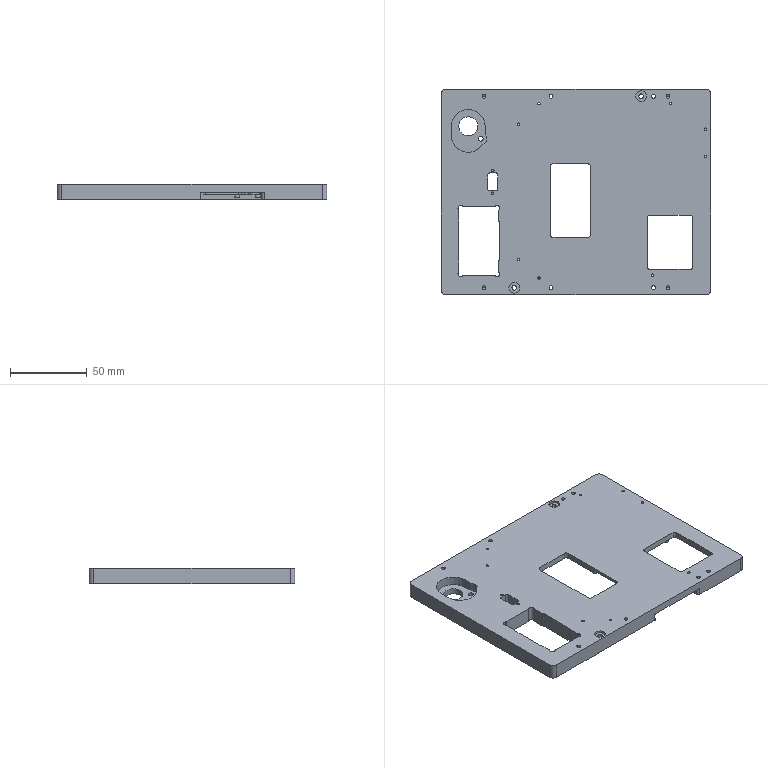NC program | NX | posted with a generic post | part box 176 x 134 x 10 mm
Lines 2298 to 3227 of 17594:
(CAVITY_MILL_COPY , TOOL : D6JING)
N4582 T16 M6
N4584 G54
N4586 G17 G0 G90 X-60.097 Y55.438 S9500 M3
N4588 G43 Z30. H16
N4590 Z-0.2
N4592 G94 G1 X-59.947 Y56.034 F1000.
N4594 G3 X-60.221 Y56.996 R1.
N4596 G2 X-60.891 Y57.969 R3. F1800.
N4598 G3 X-62.639 Y58.134 R1.
N4600 G2 X-63.497 Y57.187 R4.5
N4602 G3 X-63.844 Y56.25 R1.
N4604 G1 X-63.733 Y55.597
N4606 G0 X-60.097 Y55.438 Z-0.633
N4608 G1 X-59.947 Y56.034 F1000.
N4610 G3 X-60.221 Y56.996 R1.
N4612 G2 X-60.891 Y57.969 R3. F1800.
N4614 G3 X-62.639 Y58.134 R1.
N4616 G2 X-63.497 Y57.187 R4.5
N4618 G3 X-63.844 Y56.25 R1.
N4620 G1 X-63.733 Y55.597
N4622 G0 X-60.097 Y55.438 Z-1.067
N4624 G1 X-59.947 Y56.034 F1000.
N4626 G3 X-60.221 Y56.996 R1.
N4628 G2 X-60.891 Y57.969 R3. F1800.
N4630 G3 X-62.639 Y58.134 R1.
N4632 G2 X-63.497 Y57.187 R4.5
N4634 G3 X-63.844 Y56.25 R1.
N4636 G1 X-63.733 Y55.597
N4638 G0 X-60.097 Y55.438 Z-1.5
N4640 G1 X-59.947 Y56.034 F1000.
N4642 G3 X-60.221 Y56.996 R1.
N4644 G2 X-60.891 Y57.969 R3. F1800.
N4646 G3 X-62.639 Y58.134 R1.
N4648 G2 X-63.497 Y57.187 R4.5
N4650 G3 X-63.844 Y56.25 R1.
N4652 G1 X-63.733 Y55.597
N4654 G0 X-60.131 Y54.951 Z-1.9
N4656 G1 X-60.416 Y55.588 F1000.
N4658 G3 X-61.225 Y56.175 R1.
N4660 G2 X-61.81 Y56.275 R4.5 F1800.
N4662 X-62.395 Y56.175 R4.5
N4664 G3 X-63.205 Y55.588 R1.
N4666 G1 X-63.49 Y54.951
N4668 G0 X-60.131 Z-2.3
N4670 G1 X-60.416 Y55.588 F1000.
N4672 G3 X-61.225 Y56.175 R1.
N4674 G2 X-61.81 Y56.275 R4.5 F1800.
N4676 X-62.395 Y56.175 R4.5
N4678 G3 X-63.205 Y55.588 R1.
N4680 G1 X-63.49 Y54.951
N4682 G0 X-60.131 Z-2.7
N4684 G1 X-60.416 Y55.588 F1000.
N4686 G3 X-61.225 Y56.175 R1.
N4688 G2 X-61.81 Y56.275 R4.5 F1800.
N4690 X-62.395 Y56.175 R4.5
N4692 G3 X-63.205 Y55.588 R1.
N4694 G1 X-63.49 Y54.951
N4696 G0 X-60.131 Z-3.1
N4698 G1 X-60.416 Y55.588 F1000.
N4700 G3 X-61.225 Y56.175 R1.
N4702 G2 X-61.81 Y56.275 R4.5 F1800.
N4704 X-62.395 Y56.175 R4.5
N4706 G3 X-63.205 Y55.588 R1.
N4708 G1 X-63.49 Y54.951
N4710 G0 Z30.
N4712 X-71.161
N4714 Z-0.2
N4716 G1 X-71.565 Y55.651 F1000.
N4718 G3 X-72.431 Y56.151 R1.
N4720 G1 X-74.245 F1800.
N4722 G2 X-74.621 Y54.605 R4.5
N4724 G3 X-74.513 Y53.611 R1.
N4726 G1 X-74.123 Y53.077
N4728 G0 X-71.161 Y54.951 Z-0.633
N4730 G1 X-71.565 Y55.651 F1000.
N4732 G3 X-72.431 Y56.151 R1.
N4734 G1 X-74.245 F1800.
N4736 G2 X-74.621 Y54.605 R4.5
N4738 G3 X-74.513 Y53.611 R1.
N4740 G1 X-74.123 Y53.077
N4742 G0 X-71.161 Y54.951 Z-1.067
N4744 G1 X-71.565 Y55.651 F1000.
N4746 G3 X-72.431 Y56.151 R1.
N4748 G1 X-74.245 F1800.
N4750 G2 X-74.621 Y54.605 R4.5
N4752 G3 X-74.513 Y53.611 R1.
N4754 G1 X-74.123 Y53.077
N4756 G0 X-71.161 Y54.951 Z-1.5
N4758 G1 X-71.565 Y55.651 F1000.
N4760 G3 X-72.431 Y56.151 R1.
N4762 G1 X-74.245 F1800.
N4764 G2 X-74.621 Y54.605 R4.5
N4766 G3 X-74.513 Y53.611 R1.
N4768 G1 X-74.123 Y53.077
N4770 G0 X-71.161 Y54.951 Z-1.9
N4772 G1 X-71.565 Y55.651 F1000.
N4774 G3 X-72.431 Y56.151 R1.
N4776 G1 X-74.245 F1800.
N4778 G2 X-74.621 Y54.605 R4.5
N4780 G3 X-74.513 Y53.611 R1.
N4782 G1 X-74.123 Y53.077
N4784 G0 X-71.161 Y54.951 Z-2.3
N4786 G1 X-71.565 Y55.651 F1000.
N4788 G3 X-72.431 Y56.151 R1.
N4790 G1 X-74.245 F1800.
N4792 G2 X-74.621 Y54.605 R4.5
N4794 G3 X-74.513 Y53.611 R1.
N4796 G1 X-74.123 Y53.077
N4798 G0 X-71.161 Y54.951 Z-2.7
N4800 G1 X-71.565 Y55.651 F1000.
N4802 G3 X-72.431 Y56.151 R1.
N4804 G1 X-74.245 F1800.
N4806 G2 X-74.621 Y54.605 R4.5
N4808 G3 X-74.513 Y53.611 R1.
N4810 G1 X-74.123 Y53.077
N4812 G0 X-71.161 Y54.951 Z-3.1
N4814 G1 X-71.565 Y55.651 F1000.
N4816 G3 X-72.431 Y56.151 R1.
N4818 G1 X-74.245 F1800.
N4820 G2 X-74.621 Y54.605 R4.5
N4822 G3 X-74.513 Y53.611 R1.
N4824 G1 X-74.123 Y53.077
N4826 G0 Z30.
N4828 X-78.004 Y48.437
N4830 Z-3.6
N4832 G1 X-77.304 Y48.841 F1000.
N4834 G3 X-76.804 Y49.707 R1.
N4836 G1 Y51.924 F1800.
N4838 X-79.02
N4840 G3 X-79.886 Y51.424 R1.
N4842 G1 X-80.29 Y50.724
N4844 G0 X-78.004 Y48.437 Z-4.1
N4846 G1 X-77.304 Y48.841 F1000.
N4848 G3 X-76.804 Y49.707 R1.
N4850 G1 Y51.924 F1800.
N4852 X-79.02
N4854 G3 X-79.886 Y51.424 R1.
N4856 G1 X-80.29 Y50.724
N4858 G0 X-78.004 Y48.437 Z-4.6
N4860 G1 X-77.304 Y48.841 F1000.
N4862 G3 X-76.804 Y49.707 R1.
N4864 G1 Y51.924 F1800.
N4866 X-79.02
N4868 G3 X-79.886 Y51.424 R1.
N4870 G1 X-80.29 Y50.724
N4872 G0 Z30.
N4874 X-78.004 Y48.437
N4876 Z-5.
N4878 G1 X-77.304 Y48.841 F1000.
N4880 G3 X-76.804 Y49.707 R1.
N4882 G1 Y51.924 F1800.
N4884 X-79.02
N4886 G3 X-79.886 Y51.424 R1.
N4888 G1 X-80.29 Y50.724
N4890 G0 Z30.
N4892 X-65.182 Y42.466
N4894 Z-1.6
N4896 G1 Y49.136 Z-1.95 F1000.
N4898 X-68.438 Z-2.12
N4900 Y40.447 Z-2.576
N4902 X-65.182 Z-2.746
N4904 Y49.136 Z-3.202
N4906 X-68.438 Z-3.372
N4908 Y44.792 Z-3.6
N4910 Y40.447 F1800.
N4912 X-65.182
N4914 Y49.136
N4916 X-68.438
N4918 Y44.792
N4920 G3 X-67.938 Y43.926 R1.
N4922 G0 X-65.182 Y42.466 Z-2.1
N4924 G1 Y49.136 Z-2.45 F1000.
N4926 X-68.438 Z-2.62
N4928 Y40.447 Z-3.076
N4930 X-65.182 Z-3.246
N4932 Y49.136 Z-3.702
N4934 X-68.438 Z-3.872
N4936 Y44.792 Z-4.1
N4938 Y40.447 F1800.
N4940 X-65.182
N4942 Y49.136
N4944 X-68.438
N4946 Y44.792
N4948 G3 X-67.938 Y43.926 R1.
N4950 G0 X-65.182 Y42.466 Z-2.6
N4952 G1 Y49.136 Z-2.95 F1000.
N4954 X-68.438 Z-3.12
N4956 Y40.447 Z-3.576
N4958 X-65.182 Z-3.746
N4960 Y49.136 Z-4.202
N4962 X-68.438 Z-4.372
N4964 Y44.792 Z-4.6
N4966 Y40.447 F1800.
N4968 X-65.182
N4970 Y49.136
N4972 X-68.438
N4974 Y44.792
N4976 G3 X-67.938 Y43.926 R1.
N4978 G0 Z30.
N4980 X-65.182 Y44.374
N4982 Z-3.1
N4984 G1 Y49.136 Z-3.35 F1000.
N4986 X-68.438 Z-3.52
N4988 Y40.447 Z-3.976
N4990 X-65.182 Z-4.146
N4992 Y49.136 Z-4.602
N4994 X-68.438 Z-4.772
N4996 Y44.792 Z-5.
N4998 Y40.447 F1800.
N5000 X-65.182
N5002 Y49.136
N5004 X-68.438
N5006 Y44.792
N5008 G3 X-67.938 Y43.926 R1.
N5010 G0 X-66.144 Y49.136 Z-3.5
N5012 G1 X-68.438 Z-3.62 F1000.
N5014 Y40.447 Z-4.076
N5016 X-65.182 Z-4.246
N5018 Y49.136 Z-4.702
N5020 X-68.438 Z-4.872
N5022 Y44.792 Z-5.1
N5024 Y40.447 F1800.
N5026 X-65.182
N5028 Y49.136
N5030 X-68.438
N5032 Y44.792
N5034 G3 X-67.938 Y43.926 R1.
N5036 G0 X-65.182 Y42.466 Z-3.6
N5038 G1 Y49.136 Z-3.95 F1000.
N5040 X-68.438 Z-4.12
N5042 Y40.447 Z-4.576
N5044 X-65.182 Z-4.746
N5046 Y49.136 Z-5.202
N5048 X-68.438 Z-5.372
N5050 Y44.792 Z-5.6
N5052 Y40.447 F1800.
N5054 X-65.182
N5056 Y49.136
N5058 X-68.438
N5060 Y44.792
N5062 G3 X-67.938 Y43.926 R1.
N5064 G0 X-65.182 Y42.466 Z-4.1
N5066 G1 Y49.136 Z-4.45 F1000.
N5068 X-68.438 Z-4.62
N5070 Y40.447 Z-5.076
N5072 X-65.182 Z-5.246
N5074 Y49.136 Z-5.702
N5076 X-68.438 Z-5.872
N5078 Y44.792 Z-6.1
N5080 Y40.447 F1800.
N5082 X-65.182
N5084 Y49.136
N5086 X-68.438
N5088 Y44.792
N5090 G3 X-67.938 Y43.926 R1.
N5092 G0 Z30.
N5094 X-70.75 Y24.576
N5096 Z-5.1
N5098 G1 X-71.154 Y25.276 F1000.
N5100 G3 X-72.02 Y25.776 R1.
N5102 G1 X-74.237 F1800.
N5104 Y23.559
N5106 G3 X-73.737 Y22.693 R1.
N5108 G1 X-73.037 Y22.289
N5110 G0 X-70.75 Y24.576 Z-5.6
N5112 G1 X-71.154 Y25.276 F1000.
N5114 G3 X-72.02 Y25.776 R1.
N5116 G1 X-74.237 F1800.
N5118 Y23.559
N5120 G3 X-73.737 Y22.693 R1.
N5122 G1 X-73.037 Y22.289
N5124 G0 X-70.75 Y24.576 Z-6.1
N5126 G1 X-71.154 Y25.276 F1000.
N5128 G3 X-72.02 Y25.776 R1.
N5130 G1 X-74.237 F1800.
N5132 Y23.559
N5134 G3 X-73.737 Y22.693 R1.
N5136 G1 X-73.037 Y22.289
N5138 G0 Z30.
N5140 X-59.737 Y20.207
N5142 Z-6.6
N5144 G1 X-60.437 Y19.803 F1000.
N5146 G3 X-60.937 Y18.937 R1.
N5148 G1 Y16.72 F1800.
N5150 X-58.721
N5152 G3 X-57.854 Y17.22 R1.
N5154 G1 X-57.45 Y17.92
N5156 G0 X-59.737 Y20.207 Z-7.1
N5158 G1 X-60.437 Y19.803 F1000.
N5160 G3 X-60.937 Y18.937 R1.
N5162 G1 Y16.72 F1800.
N5164 X-58.721
N5166 G3 X-57.854 Y17.22 R1.
N5168 G1 X-57.45 Y17.92
N5170 G0 X-59.737 Y20.207 Z-7.6
N5172 G1 X-60.437 Y19.803 F1000.
N5174 G3 X-60.937 Y18.937 R1.
N5176 G1 Y16.72 F1800.
N5178 X-58.721
N5180 G3 X-57.854 Y17.22 R1.
N5182 G1 X-57.45 Y17.92
N5184 G0 X-59.737 Y20.207 Z-8.1
N5186 G1 X-60.437 Y19.803 F1000.
N5188 G3 X-60.937 Y18.937 R1.
N5190 G1 Y16.72 F1800.
N5192 X-58.721
N5194 G3 X-57.854 Y17.22 R1.
N5196 G1 X-57.45 Y17.92
N5198 G0 Z30.
N5200 X-58.758 Y27.041
N5202 Z-3.6
N5204 G1 X-59.162 Y27.741 F1000.
N5206 G3 X-60.028 Y28.241 R1.
N5208 G1 X-61.327 F1800.
N5210 G2 X-61.983 Y27.28 R4.5
N5212 G3 X-62.186 Y26.301 R1.
N5214 G1 X-61.979 Y25.673
N5216 G0 X-58.758 Y27.041 Z-4.1
N5218 G1 X-59.162 Y27.741 F1000.
N5220 G3 X-60.028 Y28.241 R1.
N5222 G1 X-61.327 F1800.
N5224 G2 X-61.983 Y27.28 R4.5
N5226 G3 X-62.186 Y26.301 R1.
N5228 G1 X-61.979 Y25.673
N5230 G0 X-58.758 Y27.041 Z-4.6
N5232 G1 X-59.162 Y27.741 F1000.
N5234 G3 X-60.028 Y28.241 R1.
N5236 G1 X-61.327 F1800.
N5238 G2 X-61.983 Y27.28 R4.5
N5240 G3 X-62.186 Y26.301 R1.
N5242 G1 X-61.979 Y25.673
N5244 G0 Z30.
N5246 X-58.758 Y27.041
N5248 Z-5.
N5250 G1 X-59.162 Y27.741 F1000.
N5252 G3 X-60.028 Y28.241 R1.
N5254 G1 X-61.327 F1800.
N5256 G2 X-61.983 Y27.28 R4.5
N5258 G3 X-62.186 Y26.301 R1.
N5260 G1 X-61.979 Y25.673
N5262 G0 X-58.758 Y27.041 Z-5.1
N5264 G1 X-59.162 Y27.741 F1000.
N5266 G3 X-60.028 Y28.241 R1.
N5268 G1 X-61.327 F1800.
N5270 G2 X-61.983 Y27.28 R4.5
N5272 G3 X-62.186 Y26.301 R1.
N5274 G1 X-61.979 Y25.673
N5276 G0 X-58.758 Y27.041 Z-5.6
N5278 G1 X-59.162 Y27.741 F1000.
N5280 G3 X-60.028 Y28.241 R1.
N5282 G1 X-61.327 F1800.
N5284 G2 X-61.983 Y27.28 R4.5
N5286 G3 X-62.186 Y26.301 R1.
N5288 G1 X-61.979 Y25.673
N5290 G0 X-58.758 Y27.041 Z-6.1
N5292 G1 X-59.162 Y27.741 F1000.
N5294 G3 X-60.028 Y28.241 R1.
N5296 G1 X-61.327 F1800.
N5298 G2 X-61.983 Y27.28 R4.5
N5300 G3 X-62.186 Y26.301 R1.
N5302 G1 X-61.979 Y25.673
N5304 G0 Z30.
N5306 X-57.45 Y27.041
N5308 Z-6.6
N5310 G1 X-57.854 Y27.741 F1000.
N5312 G3 X-58.721 Y28.241 R1.
N5314 G1 X-60.937 F1800.
N5316 Y26.024
N5318 G3 X-60.437 Y25.158 R1.
N5320 G1 X-59.737 Y24.754
N5322 G0 X-57.45 Y27.041 Z-7.1
N5324 G1 X-57.854 Y27.741 F1000.
N5326 G3 X-58.721 Y28.241 R1.
N5328 G1 X-60.937 F1800.
N5330 Y26.024
N5332 G3 X-60.437 Y25.158 R1.
N5334 G1 X-59.737 Y24.754
N5336 G0 X-57.45 Y27.041 Z-7.6
N5338 G1 X-57.854 Y27.741 F1000.
N5340 G3 X-58.721 Y28.241 R1.
N5342 G1 X-60.937 F1800.
N5344 Y26.024
N5346 G3 X-60.437 Y25.158 R1.
N5348 G1 X-59.737 Y24.754
N5350 G0 X-57.45 Y27.041 Z-8.1
N5352 G1 X-57.854 Y27.741 F1000.
N5354 G3 X-58.721 Y28.241 R1.
N5356 G1 X-60.937 F1800.
N5358 Y26.024
N5360 G3 X-60.437 Y25.158 R1.
N5362 G1 X-59.737 Y24.754
N5364 G0 Z30.
N5366 X-34.183 Y50.748
N5368 Z-3.6
N5370 G1 X-34.587 Y51.448 F1000.
N5372 G3 X-35.453 Y51.948 R1.
N5374 G1 X-37.67 F1800.
N5376 Y49.731
N5378 G3 X-37.17 Y48.865 R1.
N5380 G1 X-36.47 Y48.461
N5382 G0 X-34.183 Y50.748 Z-4.1
N5384 G1 X-34.587 Y51.448 F1000.
N5386 G3 X-35.453 Y51.948 R1.
N5388 G1 X-37.67 F1800.
N5390 Y49.731
N5392 G3 X-37.17 Y48.865 R1.
N5394 G1 X-36.47 Y48.461
N5396 G0 X-34.183 Y50.748 Z-4.6
N5398 G1 X-34.587 Y51.448 F1000.
N5400 G3 X-35.453 Y51.948 R1.
N5402 G1 X-37.67 F1800.
N5404 Y49.731
N5406 G3 X-37.17 Y48.865 R1.
N5408 G1 X-36.47 Y48.461
N5410 G0 Z30.
N5412 X-34.183 Y50.748
N5414 Z-5.
N5416 G1 X-34.587 Y51.448 F1000.
N5418 G3 X-35.453 Y51.948 R1.
N5420 G1 X-37.67 F1800.
N5422 Y49.731
N5424 G3 X-37.17 Y48.865 R1.
N5426 G1 X-36.47 Y48.461
N5428 G0 X-34.183 Y50.748 Z-5.1
N5430 G1 X-34.587 Y51.448 F1000.
N5432 G3 X-35.453 Y51.948 R1.
N5434 G1 X-37.67 F1800.
N5436 Y49.731
N5438 G3 X-37.17 Y48.865 R1.
N5440 G1 X-36.47 Y48.461
N5442 G0 X-34.183 Y50.748 Z-5.6
N5444 G1 X-34.587 Y51.448 F1000.
N5446 G3 X-35.453 Y51.948 R1.
N5448 G1 X-37.67 F1800.
N5450 Y49.731
N5452 G3 X-37.17 Y48.865 R1.
N5454 G1 X-36.47 Y48.461
N5456 G0 X-34.183 Y50.748 Z-6.1
N5458 G1 X-34.587 Y51.448 F1000.
N5460 G3 X-35.453 Y51.948 R1.
N5462 G1 X-37.67 F1800.
N5464 Y49.731
N5466 G3 X-37.17 Y48.865 R1.
N5468 G1 X-36.47 Y48.461
N5470 G0 X-34.183 Y50.748 Z-6.6
N5472 G1 X-34.587 Y51.448 F1000.
N5474 G3 X-35.453 Y51.948 R1.
N5476 G1 X-37.67 F1800.
N5478 Y49.731
N5480 G3 X-37.17 Y48.865 R1.
N5482 G1 X-36.47 Y48.461
N5484 G0 X-34.183 Y50.748 Z-7.1
N5486 G1 X-34.587 Y51.448 F1000.
N5488 G3 X-35.453 Y51.948 R1.
N5490 G1 X-37.67 F1800.
N5492 Y49.731
N5494 G3 X-37.17 Y48.865 R1.
N5496 G1 X-36.47 Y48.461
N5498 G0 X-34.183 Y50.748 Z-7.6
N5500 G1 X-34.587 Y51.448 F1000.
N5502 G3 X-35.453 Y51.948 R1.
N5504 G1 X-37.67 F1800.
N5506 Y49.731
N5508 G3 X-37.17 Y48.865 R1.
N5510 G1 X-36.47 Y48.461
N5512 G0 X-34.183 Y50.748 Z-8.1
N5514 G1 X-34.587 Y51.448 F1000.
N5516 G3 X-35.453 Y51.948 R1.
N5518 G1 X-37.67 F1800.
N5520 Y49.731
N5522 G3 X-37.17 Y48.865 R1.
N5524 G1 X-36.47 Y48.461
N5526 G0 Z30.
N5528 X-9.517
N5530 Z-3.6
N5532 G1 X-8.817 Y48.865 F1000.
N5534 G3 X-8.317 Y49.731 R1.
N5536 G1 Y51.948 F1800.
N5538 X-10.534
N5540 G3 X-11.4 Y51.448 R1.
N5542 G1 X-11.804 Y50.748
N5544 G0 X-9.517 Y48.461 Z-4.1
N5546 G1 X-8.817 Y48.865 F1000.
N5548 G3 X-8.317 Y49.731 R1.
N5550 G1 Y51.948 F1800.
N5552 X-10.534
N5554 G3 X-11.4 Y51.448 R1.
N5556 G1 X-11.804 Y50.748
N5558 G0 X-9.517 Y48.461 Z-4.6
N5560 G1 X-8.817 Y48.865 F1000.
N5562 G3 X-8.317 Y49.731 R1.
N5564 G1 Y51.948 F1800.
N5566 X-10.534
N5568 G3 X-11.4 Y51.448 R1.
N5570 G1 X-11.804 Y50.748
N5572 G0 Z30.
N5574 X-9.517 Y48.461
N5576 Z-5.
N5578 G1 X-8.817 Y48.865 F1000.
N5580 G3 X-8.317 Y49.731 R1.
N5582 G1 Y51.948 F1800.
N5584 X-10.534
N5586 G3 X-11.4 Y51.448 R1.
N5588 G1 X-11.804 Y50.748
N5590 G0 X-9.517 Y48.461 Z-5.1
N5592 G1 X-8.817 Y48.865 F1000.
N5594 G3 X-8.317 Y49.731 R1.
N5596 G1 Y51.948 F1800.
N5598 X-10.534
N5600 G3 X-11.4 Y51.448 R1.
N5602 G1 X-11.804 Y50.748
N5604 G0 X-9.517 Y48.461 Z-5.6
N5606 G1 X-8.817 Y48.865 F1000.
N5608 G3 X-8.317 Y49.731 R1.
N5610 G1 Y51.948 F1800.
N5612 X-10.534
N5614 G3 X-11.4 Y51.448 R1.
N5616 G1 X-11.804 Y50.748
N5618 G0 X-9.517 Y48.461 Z-6.1
N5620 G1 X-8.817 Y48.865 F1000.
N5622 G3 X-8.317 Y49.731 R1.
N5624 G1 Y51.948 F1800.
N5626 X-10.534
N5628 G3 X-11.4 Y51.448 R1.
N5630 G1 X-11.804 Y50.748
N5632 G0 X-9.517 Y48.461 Z-6.6
N5634 G1 X-8.817 Y48.865 F1000.
N5636 G3 X-8.317 Y49.731 R1.
N5638 G1 Y51.948 F1800.
N5640 X-10.534
N5642 G3 X-11.4 Y51.448 R1.
N5644 G1 X-11.804 Y50.748
N5646 G0 X-9.517 Y48.461 Z-7.1
N5648 G1 X-8.817 Y48.865 F1000.
N5650 G3 X-8.317 Y49.731 R1.
N5652 G1 Y51.948 F1800.
N5654 X-10.534
N5656 G3 X-11.4 Y51.448 R1.
N5658 G1 X-11.804 Y50.748
N5660 G0 X-9.517 Y48.461 Z-7.6
N5662 G1 X-8.817 Y48.865 F1000.
N5664 G3 X-8.317 Y49.731 R1.
N5666 G1 Y51.948 F1800.
N5668 X-10.534
N5670 G3 X-11.4 Y51.448 R1.
N5672 G1 X-11.804 Y50.748
N5674 G0 X-9.517 Y48.461 Z-8.1
N5676 G1 X-8.817 Y48.865 F1000.
N5678 G3 X-8.317 Y49.731 R1.
N5680 G1 Y51.948 F1800.
N5682 X-10.534
N5684 G3 X-11.4 Y51.448 R1.
N5686 G1 X-11.804 Y50.748
N5688 G0 Z30.
N5690 Y32.56
N5692 Z-6.6
N5694 G1 X-11.4 Y31.86 F1000.
N5696 G3 X-10.534 Y31.36 R1.
N5698 G1 X-8.317 F1800.
N5700 Y33.577
N5702 G3 X-8.817 Y34.443 R1.
N5704 G1 X-9.517 Y34.847
N5706 G0 X-11.804 Y32.56 Z-7.1
N5708 G1 X-11.4 Y31.86 F1000.
N5710 G3 X-10.534 Y31.36 R1.
N5712 G1 X-8.317 Y31.361 F1800.
N5714 Y33.577
N5716 G3 X-8.817 Y34.443 R1.
N5718 G1 X-9.517 Y34.847
N5720 G0 X-11.805 Y32.56 Z-7.6
N5722 G1 X-11.401 Y31.86 F1000.
N5724 G3 X-10.534 Y31.36 R1.
N5726 G1 X-8.317 Y31.361 F1800.
N5728 Y33.578
N5730 G3 X-8.817 Y34.444 R1.
N5732 G1 X-9.517 Y34.848
N5734 G0 X-11.805 Y32.56 Z-8.1
N5736 G1 X-11.401 Y31.86 F1000.
N5738 G3 X-10.535 Y31.36 R1.
N5740 G1 X-8.318 F1800.
N5742 X-8.317 Y31.361
N5744 Y33.578
N5746 G3 X-8.817 Y34.444 R1.
N5748 G1 X-9.517 Y34.848
N5750 G0 Z30.
N5752 X-2.941 Y14.186
N5754 Z-6.6
N5756 G1 X-3.345 Y14.886 F1000.
N5758 G3 X-4.211 Y15.386 R1.
N5760 G1 X-6.428 F1800.
N5762 Y13.169
N5764 G3 X-5.928 Y12.303 R1.
N5766 G1 X-5.228 Y11.899
N5768 G0 X-2.941 Y14.186 Z-7.1
N5770 G1 X-3.345 Y14.886 F1000.
N5772 G3 X-4.211 Y15.386 R1.
N5774 G1 X-6.428 F1800.
N5776 Y13.169
N5778 G3 X-5.928 Y12.303 R1.
N5780 G1 X-5.228 Y11.899
N5782 G0 X-2.941 Y14.186 Z-7.6
N5784 G1 X-3.345 Y14.886 F1000.
N5786 G3 X-4.211 Y15.386 R1.
N5788 G1 X-6.428 F1800.
N5790 Y13.169
N5792 G3 X-5.928 Y12.303 R1.
N5794 G1 X-5.228 Y11.899
N5796 G0 X-2.941 Y14.186 Z-8.1
N5798 G1 X-3.345 Y14.886 F1000.
N5800 G3 X-4.211 Y15.386 R1.
N5802 G1 X-6.428 F1800.
N5804 Y13.169
N5806 G3 X-5.928 Y12.303 R1.
N5808 G1 X-5.228 Y11.899
N5810 G0 X-2.941 Y14.186 Z-8.575
N5812 G1 X-3.345 Y14.886 F1000.
N5814 G3 X-4.211 Y15.386 R1.
N5816 G1 X-6.428 F1800.
N5818 Y13.169
N5820 G3 X-5.928 Y12.303 R1.
N5822 G1 X-5.228 Y11.899
N5824 G0 X-2.941 Y14.186 Z-9.05
N5826 G1 X-3.345 Y14.886 F1000.
N5828 G3 X-4.211 Y15.386 R1.
N5830 G1 X-6.428 F1800.
N5832 Y13.169
N5834 G3 X-5.928 Y12.303 R1.
N5836 G1 X-5.228 Y11.899
N5838 G0 X-2.941 Y14.186 Z-9.525
N5840 G1 X-3.345 Y14.886 F1000.
N5842 G3 X-4.211 Y15.386 R1.
N5844 G1 X-6.428 F1800.
N5846 Y13.169
N5848 G3 X-5.928 Y12.303 R1.
N5850 G1 X-5.228 Y11.899
N5852 G0 X-2.941 Y14.186 Z-10.
N5854 G1 X-3.345 Y14.886 F1000.
N5856 G3 X-4.211 Y15.386 R1.
N5858 G1 X-6.428 F1800.
N5860 Y13.169
N5862 G3 X-5.928 Y12.303 R1.
N5864 G1 X-5.228 Y11.899
N5866 G0 Z30.
N5868 X-21.643 Y5.196
N5870 Z-3.6
N5872 G1 X-20.943 Y5.6 F1000.
N5874 G3 X-20.443 Y6.466 R1.
N5876 G1 Y8.682 F1800.
N5878 X-22.66
N5880 G3 X-23.526 Y8.182 R1.
N5882 G1 X-23.93 Y7.482
N5884 G0 Z30.
N5886 X-36.484 Y17.92
N5888 Z-6.6
N5890 G1 X-36.08 Y17.22 F1000.
N5892 G3 X-35.214 Y16.72 R1.
N5894 G1 X-32.998 F1800.
N5896 Y18.937
N5898 G3 X-33.498 Y19.803 R1.
N5900 G1 X-34.198 Y20.207
N5902 G0 X-36.484 Y17.92 Z-7.1
N5904 G1 X-36.08 Y17.22 F1000.
N5906 G3 X-35.214 Y16.72 R1.
N5908 G1 X-32.998 F1800.
N5910 Y18.937
N5912 G3 X-33.498 Y19.803 R1.
N5914 G1 X-34.198 Y20.207
N5916 G0 X-36.484 Y17.92 Z-7.6
N5918 G1 X-36.08 Y17.22 F1000.
N5920 G3 X-35.214 Y16.72 R1.
N5922 G1 X-32.998 F1800.
N5924 Y18.937
N5926 G3 X-33.498 Y19.803 R1.
N5928 G1 X-34.198 Y20.207
N5930 G0 X-36.484 Y17.92 Z-8.1
N5932 G1 X-36.08 Y17.22 F1000.
N5934 G3 X-35.214 Y16.72 R1.
N5936 G1 X-32.998 F1800.
N5938 Y18.937
N5940 G3 X-33.498 Y19.803 R1.
N5942 G1 X-34.198 Y20.207
N5944 G0 Z30.
N5946 X-24.457 Y7.482
N5948 Z-3.6
N5950 G1 X-24.861 Y8.182 F1000.
N5952 G3 X-25.727 Y8.682 R1.
N5954 G1 X-27.943 F1800.
N5956 Y6.466
N5958 G3 X-27.443 Y5.6 R1.
N5960 G1 X-26.743 Y5.196
N5962 G0 Z30.
N5964 X-23.93 Y1.382
N5966 Z-3.6
N5968 G1 X-23.526 Y0.682 F1000.
N5970 G3 X-22.66 Y0.182 R1.
N5972 G1 X-20.443 F1800.
N5974 Y2.399
N5976 G3 X-20.943 Y3.265 R1.
N5978 G1 X-21.643 Y3.669
N5980 G0 Z30.
N5982 X-26.743
N5984 Z-3.6
N5986 G1 X-27.443 Y3.265 F1000.
N5988 G3 X-27.943 Y2.399 R1.
N5990 G1 Y0.182 F1800.
N5992 X-25.727
N5994 G3 X-24.861 Y0.682 R1.
N5996 G1 X-24.457 Y1.382
N5998 G0 X-23.369 Y4.468 Z-2.1
N6000 G1 X-22.802 Y4.852 Z-2.136 F1000.
N6002 X-22.136 Y5.13 Z-2.174
N6004 X-21.429 Y5.27 Z-2.212
N6006 X-20.707 Y5.267 Z-2.249
N6008 X-20.443 Y5.219 Z-2.263
N6010 Y8.682 Z-2.445
N6012 X-24.701 Z-2.668
N6014 X-24.646 Y8.419 Z-2.682
N6016 X-24.625 Y8.214 Z-2.693
N6018 X-24.626 Y7.677 Z-2.721
N6020 X-24.743 Y6.996 Z-2.757
N6022 X-24.989 Y6.349 Z-2.794
N6024 X-25.353 Y5.762 Z-2.83
N6026 X-25.823 Y5.254 Z-2.866
N6028 X-26.38 Y4.845 Z-2.902
N6030 X-27.006 Y4.551 Z-2.938
N6032 X-27.676 Y4.38 Z-2.975
N6034 X-27.943 Y4.359 Z-2.989
N6036 Y0.182 Z-3.208
N6038 X-24.361 Z-3.395
N6040 X-24.472 Y0.427 Z-3.41
N6042 X-24.613 Y0.911 Z-3.436
N6044 X-24.685 Y1.41 Z-3.462
N6046 Y1.947 Z-3.49
N6048 X-24.56 Y2.657 Z-3.528
N6050 X-24.296 Y3.328 Z-3.566
N6052 X-23.903 Y3.933 Z-3.604
N6054 X-23.399 Y4.448 Z-3.642
N6056 X-22.802 Y4.852 Z-3.679
N6058 X-22.136 Y5.13 Z-3.717
N6060 X-21.429 Y5.27 Z-3.755
N6062 X-20.707 Y5.267 Z-3.793
N6064 X-20.443 Y5.219 Z-3.807
N6066 Y8.682 Z-3.988
N6068 X-22.572 Z-4.1
N6070 X-24.701 F1800.
N6072 G2 X-27.943 Y4.359 R3.6
N6074 G1 Y0.182
N6076 X-24.361
N6078 G2 X-20.443 Y5.219 R3.6
N6080 G1 Y8.682
N6082 X-22.572
N6084 G3 X-23.438 Y8.182 R1.
N6086 G0 X-23.369 Y4.468 Z-2.6
N6088 G1 X-22.802 Y4.852 Z-2.636 F1000.
N6090 X-22.136 Y5.13 Z-2.674
N6092 X-21.429 Y5.27 Z-2.712
N6094 X-20.707 Y5.267 Z-2.749
N6096 X-20.443 Y5.219 Z-2.763
N6098 Y8.682 Z-2.945
N6100 X-24.701 Z-3.168
N6102 X-24.646 Y8.419 Z-3.182
N6104 X-24.625 Y8.214 Z-3.193
N6106 X-24.626 Y7.677 Z-3.221
N6108 X-24.743 Y6.996 Z-3.257
N6110 X-24.989 Y6.349 Z-3.294
N6112 X-25.353 Y5.762 Z-3.33
N6114 X-25.823 Y5.254 Z-3.366
N6116 X-26.38 Y4.845 Z-3.402
N6118 X-27.006 Y4.551 Z-3.438
N6120 X-27.676 Y4.38 Z-3.475
N6122 X-27.943 Y4.359 Z-3.489
N6124 Y0.182 Z-3.708
N6126 X-24.361 Z-3.895
N6128 X-24.472 Y0.427 Z-3.91
N6130 X-24.613 Y0.911 Z-3.936
N6132 X-24.685 Y1.41 Z-3.962
N6134 Y1.947 Z-3.99
N6136 X-24.56 Y2.657 Z-4.028
N6138 X-24.296 Y3.328 Z-4.066
N6140 X-23.903 Y3.933 Z-4.104
N6142 X-23.399 Y4.448 Z-4.142
N6144 X-22.802 Y4.852 Z-4.179
N6146 X-22.136 Y5.13 Z-4.217
N6148 X-21.429 Y5.27 Z-4.255
N6150 X-20.707 Y5.267 Z-4.293
N6152 X-20.443 Y5.219 Z-4.307
N6154 Y8.682 Z-4.488
N6156 X-22.572 Z-4.6
N6158 X-24.701 F1800.
N6160 G2 X-27.943 Y4.359 R3.6
N6162 G1 Y0.182
N6164 X-24.361
N6166 G2 X-20.443 Y5.219 R3.6
N6168 G1 Y8.682
N6170 X-22.572
N6172 G3 X-23.438 Y8.182 R1.
N6174 G0 Z30.
N6176 X-21.644 Y5.228
N6178 Z-3.1
N6180 G1 X-21.429 Y5.27 Z-3.112 F1000.
N6182 X-20.707 Y5.267 Z-3.149
N6184 X-20.443 Y5.219 Z-3.163
N6186 Y8.682 Z-3.345
N6188 X-24.701 Z-3.568
N6190 X-24.646 Y8.419 Z-3.582
N6192 X-24.625 Y8.214 Z-3.593
N6194 X-24.626 Y7.677 Z-3.621
N6196 X-24.743 Y6.996 Z-3.657
N6198 X-24.989 Y6.349 Z-3.694
N6200 X-25.353 Y5.762 Z-3.73
N6202 X-25.823 Y5.254 Z-3.766
N6204 X-26.38 Y4.845 Z-3.802
N6206 X-27.006 Y4.551 Z-3.838
N6208 X-27.676 Y4.38 Z-3.875
N6210 X-27.943 Y4.359 Z-3.889
N6212 Y0.182 Z-4.108
N6214 X-24.361 Z-4.295
N6216 X-24.472 Y0.427 Z-4.31
N6218 X-24.613 Y0.911 Z-4.336
N6220 X-24.685 Y1.41 Z-4.362
N6222 Y1.947 Z-4.39
N6224 X-24.56 Y2.657 Z-4.428
N6226 X-24.296 Y3.328 Z-4.466
N6228 X-23.903 Y3.933 Z-4.504
N6230 X-23.399 Y4.448 Z-4.542
N6232 X-22.802 Y4.852 Z-4.579
N6234 X-22.136 Y5.13 Z-4.617
N6236 X-21.429 Y5.27 Z-4.655
N6238 X-20.707 Y5.267 Z-4.693
N6240 X-20.443 Y5.219 Z-4.707
N6242 Y8.682 Z-4.888
N6244 X-22.572 Z-5.
N6246 X-24.701 F1800.
N6248 G2 X-27.943 Y4.359 R3.6
N6250 G1 Y0.182
N6252 X-24.361
N6254 G2 X-20.443 Y5.219 R3.6
N6256 G1 Y8.682
N6258 X-22.572
N6260 G3 X-23.438 Y8.182 R1.
N6262 G0 X-21.495 Y8.682 Z-3.5
N6264 G1 X-24.701 Z-3.668 F1000.
N6266 X-24.646 Y8.419 Z-3.682
N6268 X-24.625 Y8.214 Z-3.693
N6270 X-24.626 Y7.677 Z-3.721
N6272 X-24.743 Y6.996 Z-3.757
N6274 X-24.989 Y6.349 Z-3.794
N6276 X-25.353 Y5.762 Z-3.83
N6278 X-25.823 Y5.254 Z-3.866
N6280 X-26.38 Y4.845 Z-3.902
N6282 X-27.006 Y4.551 Z-3.938
N6284 X-27.676 Y4.38 Z-3.975
N6286 X-27.943 Y4.359 Z-3.989
N6288 Y0.182 Z-4.208
N6290 X-24.361 Z-4.395
N6292 X-24.472 Y0.427 Z-4.41
N6294 X-24.613 Y0.911 Z-4.436
N6296 X-24.685 Y1.41 Z-4.462
N6298 Y1.947 Z-4.49
N6300 X-24.56 Y2.657 Z-4.528
N6302 X-24.296 Y3.328 Z-4.566
N6304 X-23.903 Y3.933 Z-4.604
N6306 X-23.399 Y4.448 Z-4.642
N6308 X-22.802 Y4.852 Z-4.679
N6310 X-22.136 Y5.13 Z-4.717
N6312 X-21.429 Y5.27 Z-4.755
N6314 X-20.707 Y5.267 Z-4.793
N6316 X-20.443 Y5.219 Z-4.807
N6318 Y8.682 Z-4.988
N6320 X-22.572 Z-5.1
N6322 X-24.701 F1800.
N6324 G2 X-27.943 Y4.359 R3.6
N6326 G1 Y0.182
N6328 X-24.361
N6330 G2 X-20.443 Y5.219 R3.6
N6332 G1 Y8.682
N6334 X-22.572
N6336 G3 X-23.438 Y8.182 R1.
N6338 G0 Z30.
N6340 X-36.595 Y-8.303
N6342 Z-3.6
N6344 G1 X-35.897 Y-7.901 F1000.
N6346 G3 X-35.397 Y-7.035 R1.
N6348 G1 Y-4.818 F1800.
N6350 X-37.614
N6352 G3 X-38.48 Y-5.318 R1.
N6354 G1 X-38.884 Y-6.018
N6356 G0 X-36.595 Y-8.303 Z-4.1
N6358 G1 X-35.897 Y-7.901 F1000.
N6360 G3 X-35.397 Y-7.035 R1.
N6362 G1 Y-4.818 F1800.
N6364 X-37.614
N6366 G3 X-38.48 Y-5.318 R1.
N6368 G1 X-38.884 Y-6.018
N6370 G0 X-36.595 Y-8.303 Z-4.6
N6372 G1 X-35.897 Y-7.901 F1000.
N6374 G3 X-35.397 Y-7.035 R1.
N6376 G1 Y-4.818 F1800.
N6378 X-37.614
N6380 G3 X-38.48 Y-5.318 R1.
N6382 G1 X-38.884 Y-6.018
N6384 G0 Z30.
N6386 X-30.714 Y-12.35
N6388 Z-5.
N6390 G1 X-31.118 Y-11.65 F1000.
N6392 G3 X-31.984 Y-11.15 R1.
N6394 G1 X-33.636 F1800.
N6396 G2 X-34.126 Y-12.522 R4.5
N6398 G3 X-34.107 Y-13.521 R1.
N6400 G1 X-33.046 Y-15.284
N6402 G0 X-30.714 Y-12.35 Z-5.1
N6404 G1 X-31.118 Y-11.65 F1000.
N6406 G3 X-31.984 Y-11.15 R1.
N6408 G1 X-33.636 F1800.
N6410 G2 X-34.126 Y-12.522 R4.5
N6412 G3 X-34.107 Y-13.521 R1.
N6414 G1 X-33.046 Y-15.284
N6416 G0 X-30.714 Y-12.35 Z-5.6
N6418 G1 X-31.118 Y-11.65 F1000.
N6420 G3 X-31.984 Y-11.15 R1.
N6422 G1 X-33.636 F1800.
N6424 G2 X-34.126 Y-12.522 R4.5
N6426 G3 X-34.107 Y-13.521 R1.
N6428 G1 X-33.046 Y-15.284
N6430 G0 X-30.714 Y-12.35 Z-6.1
N6432 G1 X-31.118 Y-11.65 F1000.
N6434 G3 X-31.984 Y-11.15 R1.